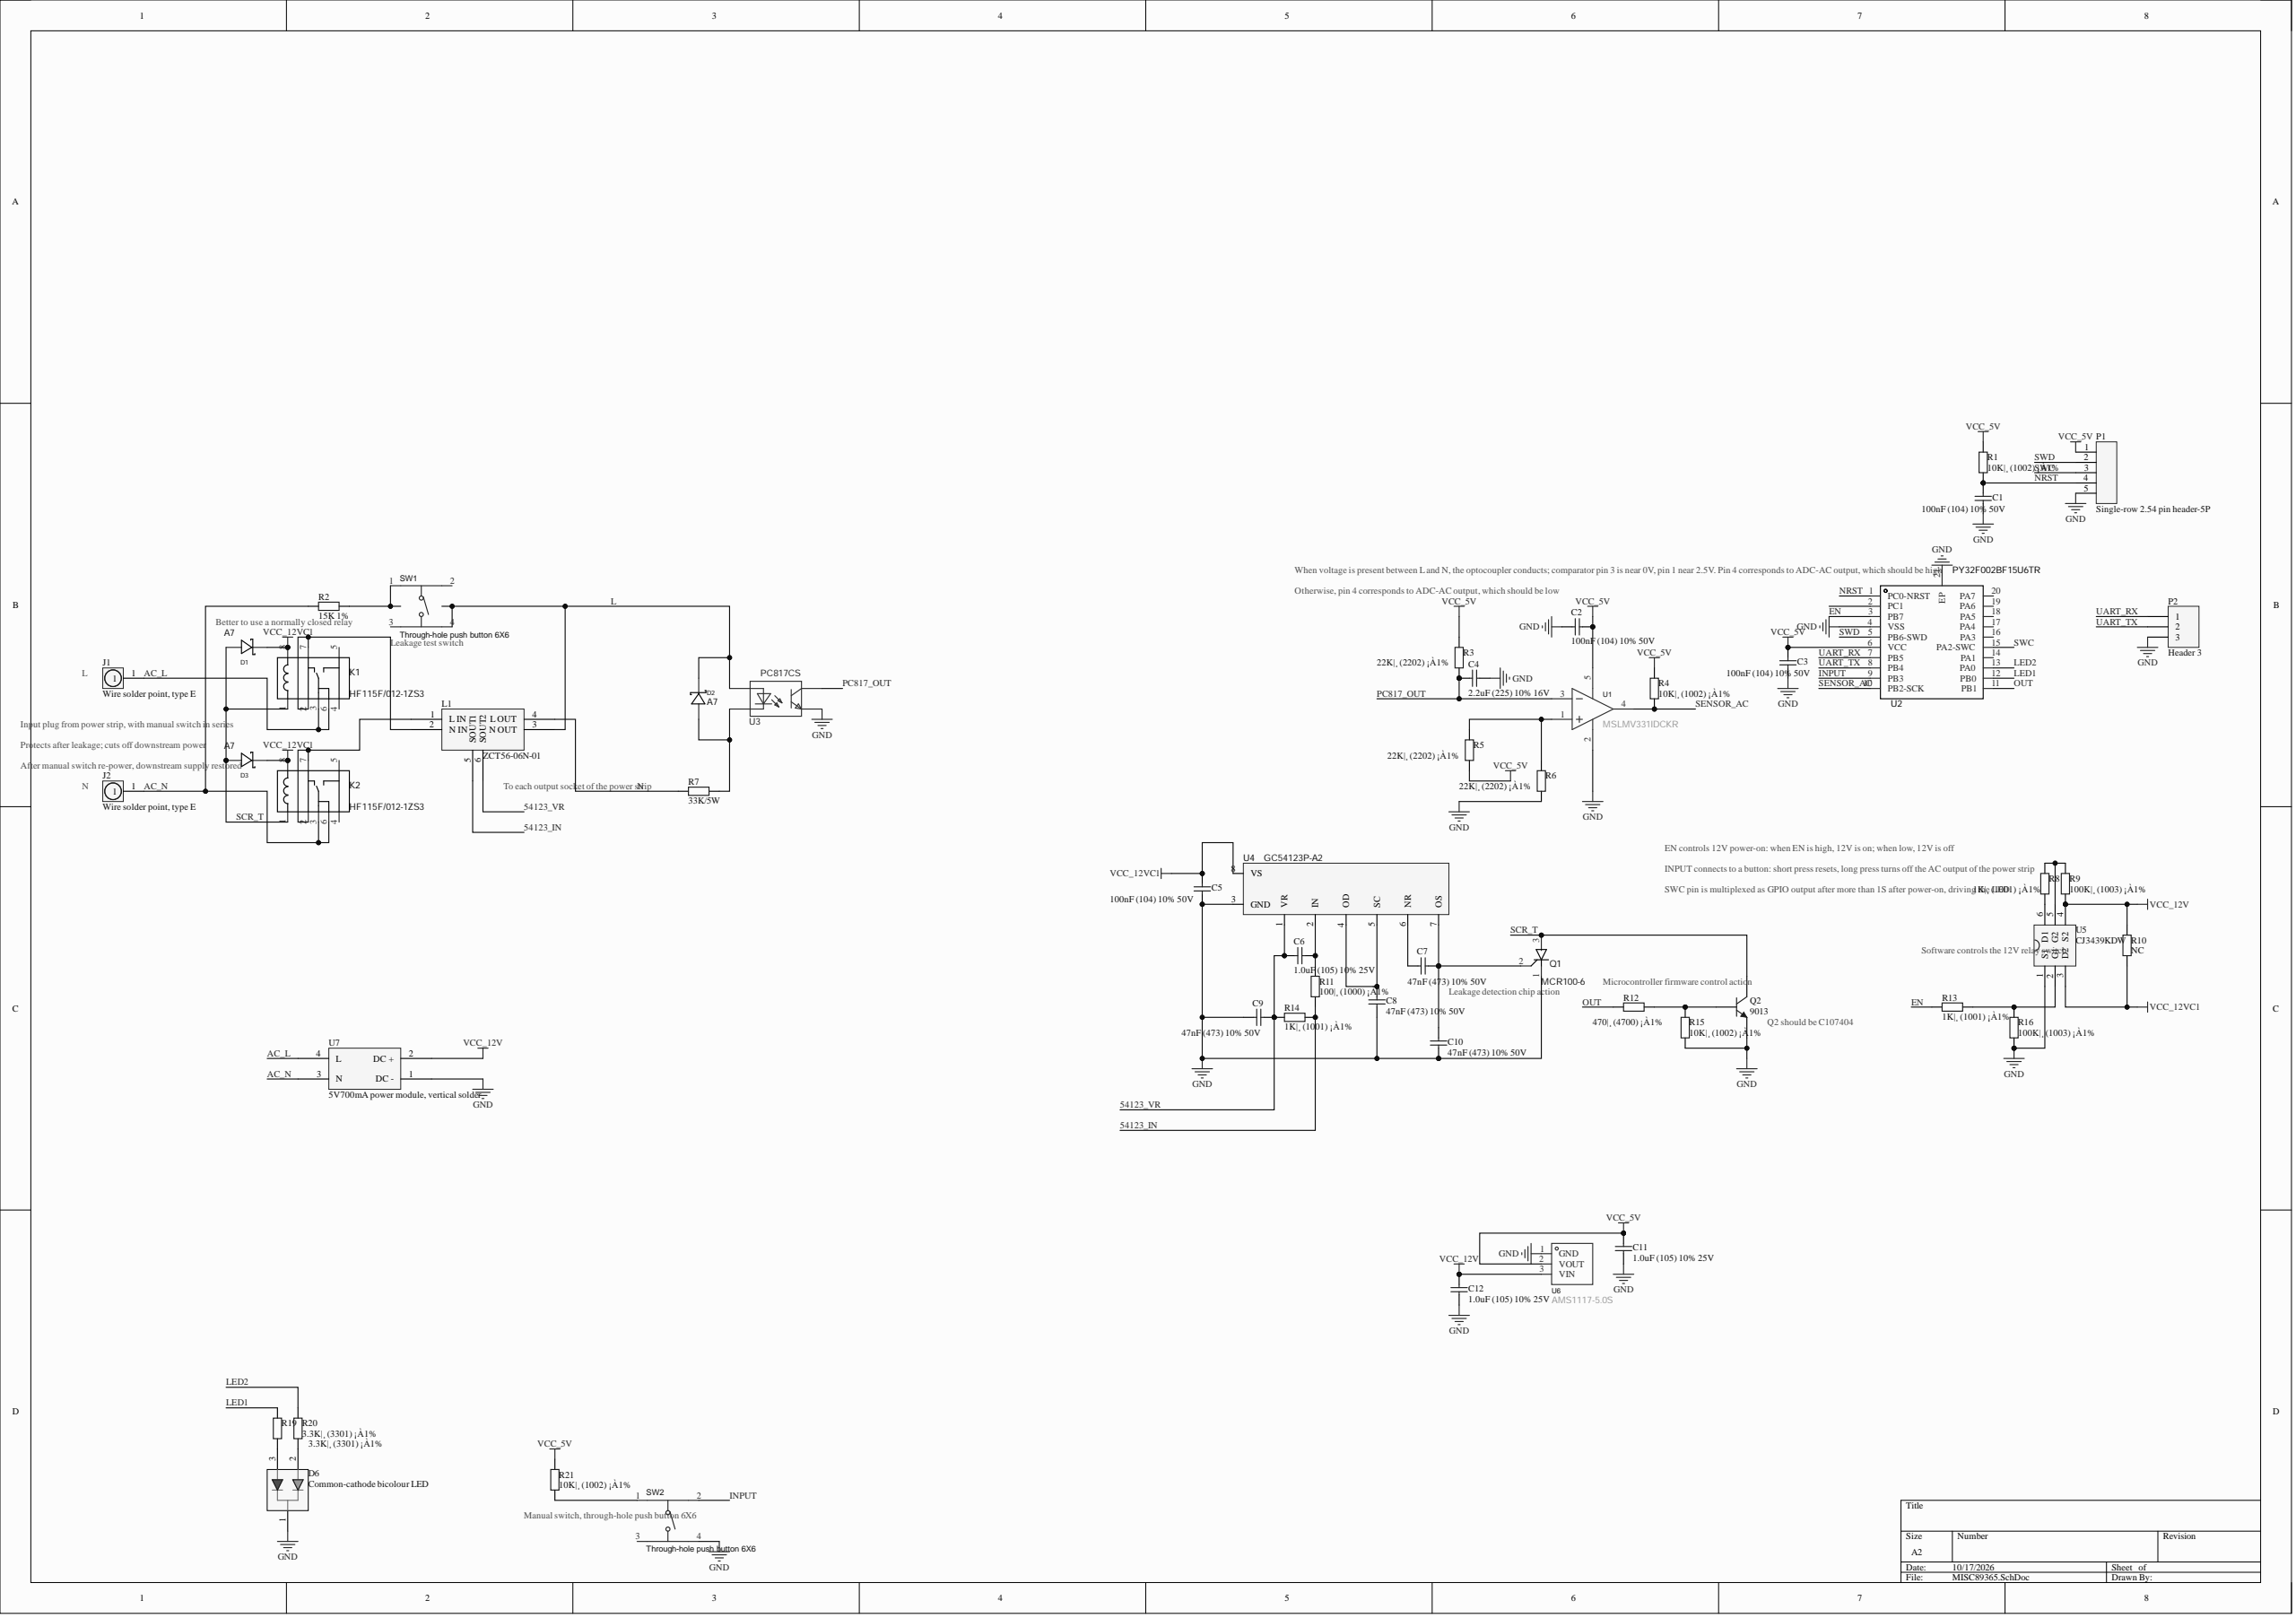Circuit board | Altium Designer | 53 parts | 39 nets
Bill of materials:
Comment,Description,Designator,Footprint,LibRef,Quantity
"100nF (104) 10% 50V","SMD capacitor","C1, C2, C3, C5","0402_C","0402 100nF (104) 10% 50V","4"
"2.2uF (225) 10% 16V","SMD capacitor","C4","0603_C","0603 2.2uF (225) 10% 16V","1"
"1.0uF (105) 10% 25V","SMD capacitor","C6, C11, C12","0402_C","0402 1.0uF (105) 10% 25V","3"
"47nF (473) 10% 50V","SMD capacitor","C7, C8, C9, C10","0402_C","0402 47nF (473) 10% 50V","4"
"A7","General-purpose diode","D1, D2, D3","SOD-123FL_L2.8-W1.8-LS3.7-RD","A7","3"
"Common-cathode bicolour LED","Bicolour LED red+green","D6","LED 3MM-2P","LED 3MM-2P共阴","1"
"Wire solder point, type E","Wire solder joint, hole diameter about 3mm","J1, J2","焊线点E型","焊线点E型","2"
"HF115F/012-1ZS3","Single changeover (SPDT)","K1, K2","RELAY-TH_HF115F-012-1ZS3","HF115F/012-1ZS3","2"
"ZCT56-06N-01","Miniature solder-pad zero-sequence sensor","L1","ZCT56-06N-01","ZCT56-06N-01","1"
"Single-row 2.54 pin header-5P","Single-row 2.54 pin header-5P","P1","HDR1X5","单排2.54排针-5P","1"
"Header 3","Header, 3-Pin","P2","HDR1X3","Header 3","1"
"MCR100-6","0.8A unidirectional thyristor","Q1","SOT-23-3_L2.9-W1.3-P1.90-LS2.4-BR","MCR100-6","1"
"9013","Transistor","Q2","SOT-23(SOT-23-3)","SOT-23 9013","1"
"10K|¸ (1002) ¡À1%","SMD resistor","R1, R4, R15, R21","0402_R","0402 10K|¸ (1002) 1%","4"
"15K 1%","SMD resistor","R2","1210_R","1210 15K 1%","1"
"22K|¸ (2202) ¡À1%","SMD resistor","R3, R5, R6","0402_R","0402 22K|¸ (2202) 1%","3"
"33K/5W","5W through-hole resistor","R7","5W直插电阻横插","33K/5W","1"
"1K|¸ (1001) ¡À1%","SMD resistor","R8, R13, R14","0402_R","0402 1K|¸ (1001) 1%","3"
"100K|¸ (1003) ¡À1%","SMD resistor","R9, R16","0402_R","0402 100K|¸ (1003) 1%","2"
"NC","SMD resistor","R10","0603_R","0603 0|¸ (0R0) 1%","1"
"100|¸ (1000) ¡À1%","SMD resistor","R11","0402_R","0402 100|¸ (1000) 1%","1"
"470|¸ (4700) ¡À1%","SMD resistor","R12","0402_R","0402 470|¸ (4700) 1%","1"
"3.3K|¸ (3301) ¡À1%","SMD resistor","R19, R20","0402_R","0402 3.3K|¸ (3301) 1%","2"
"Through-hole push button 6X6","","SW1, SW2","SW-TH_4P-L6.0-W6.0-P4.50-LS6.5","直插按键6X6","2"
"MSLMV331IDCKR","Single-channel comparator","U1","SC-70-5_L2.1-W1.3-P0.65-LS2.3-BL","MSLMV331IDCKR","1"
"PY32F002BF15U6TR","PUYA M0 microcontroller","U2","QFN-20_L3.0-W3.0-P0.40-TL-EP1.7","PY32F002BF15U6TR","1"
"PC817CS","Optocoupler","U3","SOP-4_L6.5-W4.6-P2.54-LS10.2-BL","PC817CS","1"
"GC54123P-A2","Leakage protection","U4","SOP-8_L5.0-W4.0-P1.27-LS6.2-BL","GC54123P-A2","1"
"CJ3439KDW","NMOS+PMOS","U5","SOT-363","CJ3439KDW","1"
"AMS1117-5.0S","","U6","SOT-89-3_L4.5-W2.5-P1.50-LS4.2-BR","AMS1117-5.0S","1"
"5V700mA power module, vertical solder","","U7","5V700mA电源模块竖直焊接","5V700mA电源模块竖直焊接","1"
Netlist (Protel format):
[
C1
0402_C
100nF (104) 10% 50V



]
[
C2
0402_C
100nF (104) 10% 50V



]
[
C3
0402_C
100nF (104) 10% 50V



]
[
C4
0603_C
2.2uF (225) 10% 16V



]
[
C5
0402_C
100nF (104) 10% 50V



]
[
C6
0402_C
1.0uF (105) 10% 25V



]
[
C7
0402_C
47nF (473) 10% 50V



]
[
C8
0402_C
47nF (473) 10% 50V



]
[
C9
0402_C
47nF (473) 10% 50V



]
[
C10
0402_C
47nF (473) 10% 50V



]
[
C11
0402_C
1.0uF (105) 10% 25V



]
[
C12
0402_C
1.0uF (105) 10% 25V



]
[
D1
SOD-123FL_L2.8-W1.8-LS3.7-RD
A7



]
[
D2
SOD-123FL_L2.8-W1.8-LS3.7-RD
A7



]
[
D3
SOD-123FL_L2.8-W1.8-LS3.7-RD
A7



]
[
D6
LED 3MM-2P
Common-cathode bicolour LED



]
[
J1
焊线点E型
Wire solder point, type E



]
[
J2
焊线点E型
Wire solder point, type E



]
[
K1
RELAY-TH_HF115F-012-1ZS3
HF115F/012-1ZS3



]
[
K2
RELAY-TH_HF115F-012-1ZS3
HF115F/012-1ZS3



]
[
L1
ZCT56-06N-01
ZCT56-06N-01



]
[
P1
HDR1X5
Single-row 2.54 pin header-5P



]
[
P2
HDR1X3
Header 3



]
[
Q1
SOT-23-3_L2.9-W1.3-P1.90-LS2.4-BR
MCR100-6



]
[
Q2
SOT-23(SOT-23-3)
9013



]
[
R1
0402_R
10K|¸ (1002) ¡À1%



]
[
R2
1210_R
15K 1%



]
[
R3
0402_R
22K|¸ (2202) ¡À1%



]
[
R4
0402_R
10K|¸ (1002) ¡À1%



]
[
R5
0402_R
22K|¸ (2202) ¡À1%



]
[
R6
0402_R
22K|¸ (2202) ¡À1%



]
[
R7
5W直插电阻横插
33K/5W



]
[
R8
0402_R
1K|¸ (1001) ¡À1%



]
[
R9
0402_R
100K|¸ (1003) ¡À1%



]
[
R10
0603_R
NC



]
[
R11
0402_R
100|¸ (1000) ¡À1%



]
[
R12
0402_R
470|¸ (4700) ¡À1%



]
[
R13
0402_R
1K|¸ (1001) ¡À1%



]
[
R14
0402_R
1K|¸ (1001) ¡À1%



]
[
R15
0402_R
10K|¸ (1002) ¡À1%



]
[
R16
0402_R
100K|¸ (1003) ¡À1%



]
[
R19
0402_R
3.3K|¸ (3301) ¡À1%



]
[
R20
0402_R
3.3K|¸ (3301) ¡À1%



]
[
R21
0402_R
10K|¸ (1002) ¡À1%



]
[
SW1
SW-TH_4P-L6.0-W6.0-P4.50-LS6.5
Through-hole push button 6X6



]
[
SW2
SW-TH_4P-L6.0-W6.0-P4.50-LS6.5
Through-hole push button 6X6



]
[
U1
SC-70-5_L2.1-W1.3-P0.65-LS2.3-BL
MSLMV331IDCKR



]
[
U2
QFN-20_L3.0-W3.0-P0.40-TL-EP1.7
PY32F002BF15U6TR



]
[
U3
SOP-4_L6.5-W4.6-P2.54-LS10.2-BL
PC817CS



]
[
U4
SOP-8_L5.0-W4.0-P1.27-LS6.2-BL
GC54123P-A2



]
[
U5
SOT-363
CJ3439KDW



]
[
U6
SOT-89-3_L4.5-W2.5-P1.50-LS4.2-BR
AMS1117-5.0S



]
[
U7
5V700mA电源模块竖直焊接
5V700mA power module, vertical solder



]
(
VCC_12VC1
C5-2
D1-1
D3-1
K1-8
K2-8
R10-1
U4-8
U5-3
)
(
VCC_12V
C12-2
R9-1
R10-2
U5-4
U6-3
U7-2
)
(
VCC_5V
C2-1
C3-1
C11-2
P1-1
R1-2
R3-2
R4-2
R5-1
R21-2
U1-5
U2-6
U6-2
)
(
UART_TX
P2-2
U2-8
)
(
UART_RX
P2-1
U2-7
)
(
SWD
P1-2
U2-5
)
(
SWC
P1-3
U2-15
)
(
SENSOR_AC
R4-1
U1-4
U2-10
)
(
SCR_T
D1-2
D3-2
K1-1
K2-1
Q1-3
Q2-3
)
(
PC817_OUT
C4-1
R3-1
U1-3
U3-4
)
(
OUT
R12-1
U2-11
)
(
NRST
C1-1
P1-4
R1-1
U2-1
)
(
NetR21_1
R21-1
SW2-1
)
(
NetR13_2
R13-2
R16-2
U5-2
)
(
NetR8_2
R8-2
R9-2
U5-5
)
(
NetR8_1
R8-1
U5-6
)
(
NetR5_2
R5-2
R6-2
U1-1
)
(
NetR2_2
R2-2
SW1-1
)
(
NetQ2_1
Q2-1
R12-2
R15-2
)
(
NetK2_2
K2-2
K2-7
L1-1
)
(
NetK1_2
K1-2
K1-7
L1-2
)
(
NetD6_3
D6-3
R19-1
)
(
NetD6_2
D6-2
R20-1
)
(
NetD2_2
D2-2
R7-2
U3-2
)
(
NetC8_2
C8-2
U4-4
U4-5
)
(
NetC7_2
C7-2
C10-2
Q1-2
U4-7
)
(
NetC7_1
C7-1
U4-6
)
(
NetC6_1
C6-1
R11-2
U4-2
)
(
N
L1-4
R7-1
)
(
LED2
R20-2
U2-13
)
(
LED1
R19-2
U2-12
)
(
L
D2-1
L1-3
SW1-4
U3-1
)
(
INPUT
SW2-2
U2-9
)
(
GND
C1-2
C2-2
C3-2
C4-2
C5-1
C8-1
C9-1
C10-1
C11-1
C12-1
D6-1
P1-5
P2-3
Q1-1
Q2-2
R6-1
R15-1
R16-1
SW2-4
U1-2
U2-4
U2-21
U3-3
U4-3
U5-1
U6-1
U7-1
)
(
EN
R13-1
U2-3
)
(
AC_N
J2-1
K2-3
K2-6
R2-1
U7-3
)
(
AC_L
J1-1
K1-3
K1-6
U7-4
)
(
54123_VR
C6-2
C9-2
L1-6
R14-1
U4-1
)
(
54123_IN
L1-5
R11-1
R14-2
)